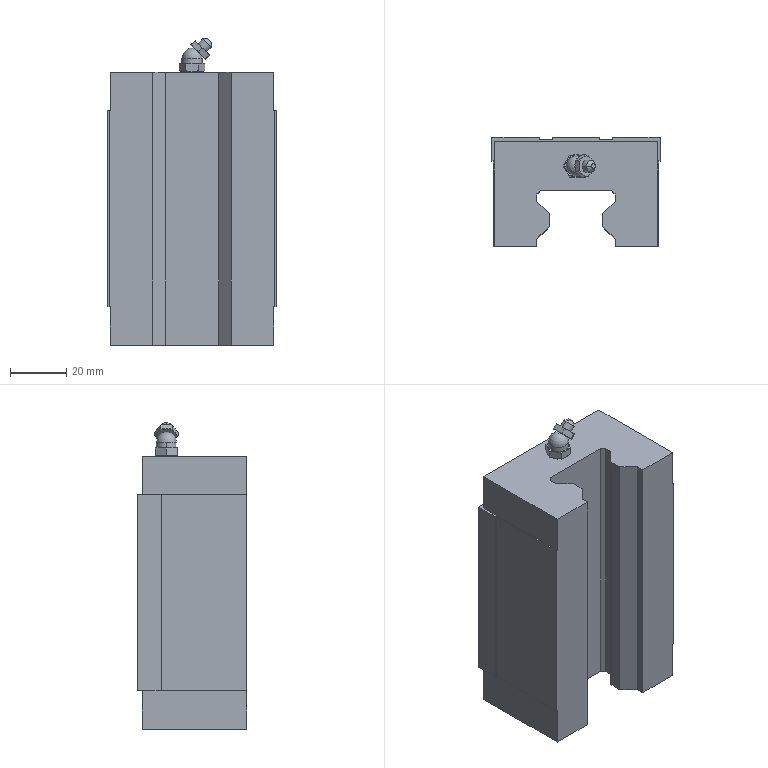Part | SolidWorks | features BaseBody 1 | 1 solid | 102 faces | box 60 x 39 x 109.4 mm | volume 173281 mm3 | plane 61 | cone 26 | cylinder 14 | sphere 1 | commonest cylinder face diameters 8 x8 7.2 x4 4.32 x2